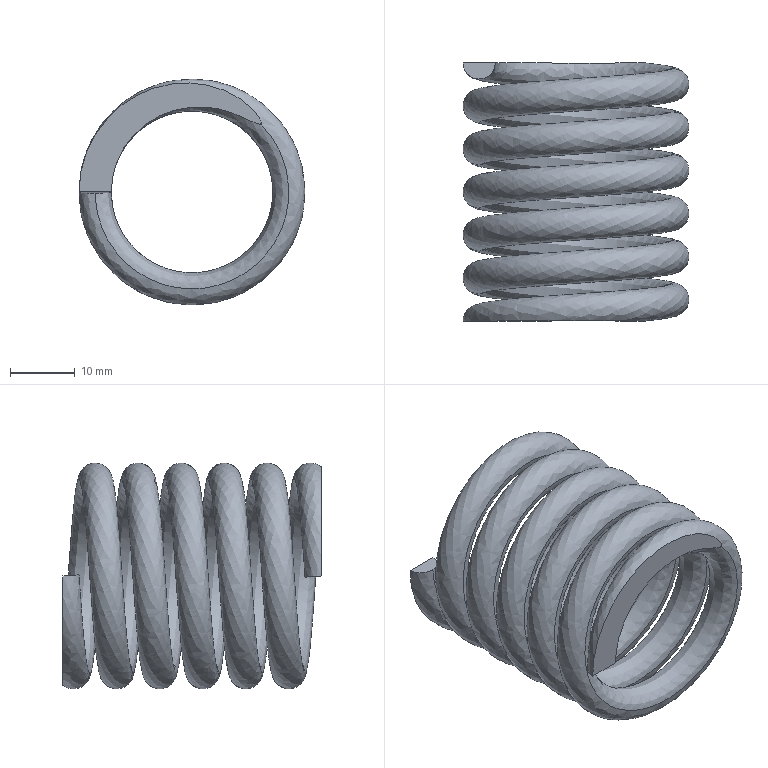Part | SolidWorks | features BaseBody 1 | 1 solid | 6 faces | volume 10843 mm3 | plane 4 | spline 2